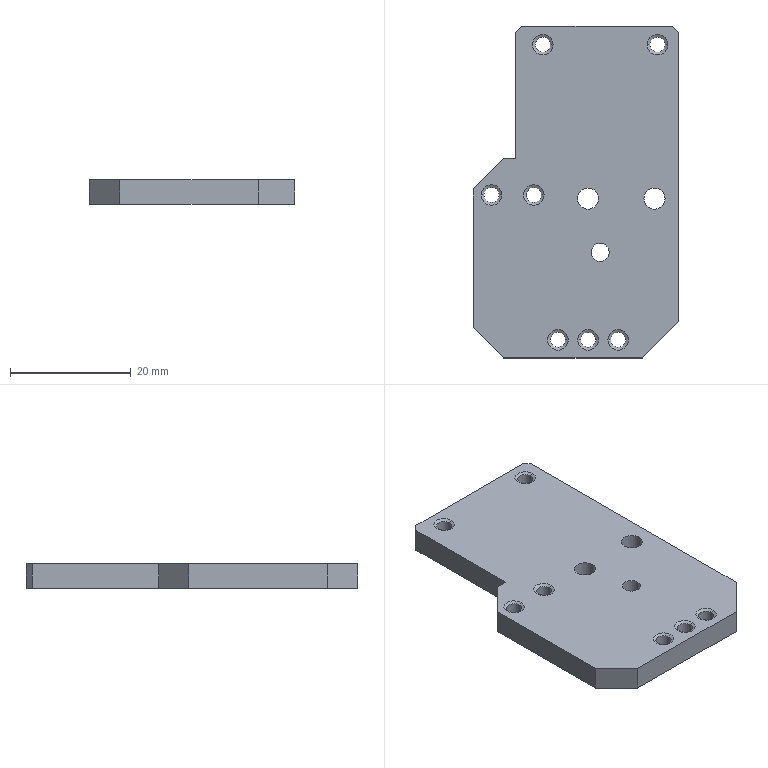Part | NX | 1 solid | 47 faces | box 34 x 55 x 4 mm | volume 6442 mm3 | cylinder 20 | cone 14 | plane 13 | commonest cylinder face diameters 2.5 x14 3.5 x4 3 x2
STEP:
#1=CARTESIAN_POINT('',(-9.5,5.5,2.));
#2=VERTEX_POINT('',#1);
#3=CARTESIAN_POINT('',(-11.5,5.5,2.));
#4=VERTEX_POINT('',#3);
#5=CARTESIAN_POINT('',(0.,5.5,2.));
#6=DIRECTION('',(-1.,0.,0.));
#7=VECTOR('',#6,1000.);
#8=LINE('',#5,#7);
#9=EDGE_CURVE('',#2,#4,#8,.T.);
#10=ORIENTED_EDGE('',*,*,#9,.T.);
#11=CARTESIAN_POINT('',(-16.5,0.5,2.));
#12=VERTEX_POINT('',#11);
#13=CARTESIAN_POINT('',(-17.,0.,2.));
#14=DIRECTION('',(-0.7071,-0.7071,0.));
#15=VECTOR('',#14,1000.);
#16=LINE('',#13,#15);
#17=EDGE_CURVE('',#4,#12,#16,.T.);
#18=ORIENTED_EDGE('',*,*,#17,.T.);
#19=CARTESIAN_POINT('',(-16.5,-22.5,2.));
#20=VERTEX_POINT('',#19);
#21=CARTESIAN_POINT('',(-16.5,0.,2.));
#22=DIRECTION('',(0.,-1.,0.));
#23=VECTOR('',#22,1000.);
#24=LINE('',#21,#23);
#25=EDGE_CURVE('',#12,#20,#24,.T.);
#26=ORIENTED_EDGE('',*,*,#25,.T.);
#27=CARTESIAN_POINT('',(-11.5,-27.5,2.));
#28=VERTEX_POINT('',#27);
#29=CARTESIAN_POINT('',(-39.,0.,2.));
#30=DIRECTION('',(-0.7071,0.7071,0.));
#31=VECTOR('',#30,1000.);
#32=LINE('',#29,#31);
#33=EDGE_CURVE('',#28,#20,#32,.T.);
#34=ORIENTED_EDGE('',*,*,#33,.F.);
#35=CARTESIAN_POINT('',(11.5,-27.5,2.));
#36=VERTEX_POINT('',#35);
#37=CARTESIAN_POINT('',(0.,-27.5,2.));
#38=DIRECTION('',(-1.,0.,0.));
#39=VECTOR('',#38,1000.);
#40=LINE('',#37,#39);
#41=EDGE_CURVE('',#36,#28,#40,.T.);
#42=ORIENTED_EDGE('',*,*,#41,.F.);
#43=CARTESIAN_POINT('',(17.5,-21.5,2.));
#44=VERTEX_POINT('',#43);
#45=CARTESIAN_POINT('',(39.,0.,2.));
#46=DIRECTION('',(-0.7071,-0.7071,0.));
#47=VECTOR('',#46,1000.);
#48=LINE('',#45,#47);
#49=EDGE_CURVE('',#44,#36,#48,.T.);
#50=ORIENTED_EDGE('',*,*,#49,.F.);
#51=CARTESIAN_POINT('',(17.5,26.5,2.));
#52=VERTEX_POINT('',#51);
#53=CARTESIAN_POINT('',(17.5,0.,2.));
#54=DIRECTION('',(0.,-1.,0.));
#55=VECTOR('',#54,1000.);
#56=LINE('',#53,#55);
#57=EDGE_CURVE('',#52,#44,#56,.T.);
#58=ORIENTED_EDGE('',*,*,#57,.F.);
#59=CARTESIAN_POINT('',(16.5,27.5,2.));
#60=VERTEX_POINT('',#59);
#61=CARTESIAN_POINT('',(44.,0.,2.));
#62=DIRECTION('',(0.7071,-0.7071,0.));
#63=VECTOR('',#62,1000.);
#64=LINE('',#61,#63);
#65=EDGE_CURVE('',#60,#52,#64,.T.);
#66=ORIENTED_EDGE('',*,*,#65,.F.);
#67=CARTESIAN_POINT('',(-8.5,27.5,2.));
#68=VERTEX_POINT('',#67);
#69=CARTESIAN_POINT('',(0.,27.5,2.));
#70=DIRECTION('',(1.,0.,0.));
#71=VECTOR('',#70,1000.);
#72=LINE('',#69,#71);
#73=EDGE_CURVE('',#68,#60,#72,.T.);
#74=ORIENTED_EDGE('',*,*,#73,.F.);
#75=CARTESIAN_POINT('',(-9.5,26.5,2.));
#76=VERTEX_POINT('',#75);
#77=CARTESIAN_POINT('',(-36.,0.,2.));
#78=DIRECTION('',(-0.7071,-0.7071,0.));
#79=VECTOR('',#78,1000.);
#80=LINE('',#77,#79);
#81=EDGE_CURVE('',#68,#76,#80,.T.);
#82=ORIENTED_EDGE('',*,*,#81,.T.);
#83=CARTESIAN_POINT('',(-9.5,0.,2.));
#84=DIRECTION('',(0.,-1.,0.));
#85=VECTOR('',#84,1000.);
#86=LINE('',#83,#85);
#87=EDGE_CURVE('',#76,#2,#86,.T.);
#88=ORIENTED_EDGE('',*,*,#87,.T.);
#89=EDGE_LOOP('',(#10,#18,#26,#34,#42,#50,#58,#66,#74,#82,#88));
#90=FACE_BOUND('',#89,.T.);
#91=CARTESIAN_POINT('',(15.25,-1.1,2.));
#92=VERTEX_POINT('',#91);
#93=CARTESIAN_POINT('',(11.75,-1.1,2.));
#94=VERTEX_POINT('',#93);
#95=CARTESIAN_POINT('',(13.5,-1.1,2.));
#96=DIRECTION('',(0.,0.,1.));
#97=DIRECTION('',(1.,0.,0.));
#98=AXIS2_PLACEMENT_3D('',#95,#96,#97);
#99=CIRCLE('',#98,1.75);
#100=EDGE_CURVE('',#92,#94,#99,.T.);
#101=ORIENTED_EDGE('',*,*,#100,.F.);
#102=CARTESIAN_POINT('',(13.5,-1.1,2.));
#103=DIRECTION('',(0.,0.,1.));
#104=DIRECTION('',(1.,0.,0.));
#105=AXIS2_PLACEMENT_3D('',#102,#103,#104);
#106=CIRCLE('',#105,1.75);
#107=EDGE_CURVE('',#94,#92,#106,.T.);
#108=ORIENTED_EDGE('',*,*,#107,.F.);
#109=EDGE_LOOP('',(#101,#108));
#110=FACE_BOUND('',#109,.T.);
#111=CARTESIAN_POINT('',(0.8,-24.5,2.));
#112=VERTEX_POINT('',#111);
#113=CARTESIAN_POINT('',(4.2,-24.5,2.));
#114=VERTEX_POINT('',#113);
#115=CARTESIAN_POINT('',(2.5,-24.5,2.));
#116=DIRECTION('',(0.,0.,1.));
#117=DIRECTION('',(1.,0.,0.));
#118=AXIS2_PLACEMENT_3D('',#115,#116,#117);
#119=CIRCLE('',#118,1.7);
#120=EDGE_CURVE('',#112,#114,#119,.T.);
#121=ORIENTED_EDGE('',*,*,#120,.F.);
#122=CARTESIAN_POINT('',(2.5,-24.5,2.));
#123=DIRECTION('',(0.,0.,1.));
#124=DIRECTION('',(1.,0.,0.));
#125=AXIS2_PLACEMENT_3D('',#122,#123,#124);
#126=CIRCLE('',#125,1.7);
#127=EDGE_CURVE('',#114,#112,#126,.T.);
#128=ORIENTED_EDGE('',*,*,#127,.F.);
#129=EDGE_LOOP('',(#121,#128));
#130=FACE_BOUND('',#129,.T.);
#131=CARTESIAN_POINT('',(-11.8,-0.5,2.));
#132=VERTEX_POINT('',#131);
#133=CARTESIAN_POINT('',(-15.2,-0.5,2.));
#134=VERTEX_POINT('',#133);
#135=CARTESIAN_POINT('',(-13.5,-0.5,2.));
#136=DIRECTION('',(0.,0.,1.));
#137=DIRECTION('',(1.,0.,0.));
#138=AXIS2_PLACEMENT_3D('',#135,#136,#137);
#139=CIRCLE('',#138,1.7);
#140=EDGE_CURVE('',#132,#134,#139,.T.);
#141=ORIENTED_EDGE('',*,*,#140,.F.);
#142=CARTESIAN_POINT('',(-13.5,-0.5,2.));
#143=DIRECTION('',(0.,0.,1.));
#144=DIRECTION('',(1.,0.,0.));
#145=AXIS2_PLACEMENT_3D('',#142,#143,#144);
#146=CIRCLE('',#145,1.7);
#147=EDGE_CURVE('',#134,#132,#146,.T.);
#148=ORIENTED_EDGE('',*,*,#147,.F.);
#149=EDGE_LOOP('',(#141,#148));
#150=FACE_BOUND('',#149,.T.);
#151=CARTESIAN_POINT('',(-6.7,24.4,2.));
#152=VERTEX_POINT('',#151);
#153=CARTESIAN_POINT('',(-3.3,24.4,2.));
#154=VERTEX_POINT('',#153);
#155=CARTESIAN_POINT('',(-5.,24.4,2.));
#156=DIRECTION('',(0.,0.,1.));
#157=DIRECTION('',(1.,0.,0.));
#158=AXIS2_PLACEMENT_3D('',#155,#156,#157);
#159=CIRCLE('',#158,1.7);
#160=EDGE_CURVE('',#152,#154,#159,.T.);
#161=ORIENTED_EDGE('',*,*,#160,.F.);
#162=CARTESIAN_POINT('',(-5.,24.4,2.));
#163=DIRECTION('',(0.,0.,1.));
#164=DIRECTION('',(1.,0.,0.));
#165=AXIS2_PLACEMENT_3D('',#162,#163,#164);
#166=CIRCLE('',#165,1.7);
#167=EDGE_CURVE('',#154,#152,#166,.T.);
#168=ORIENTED_EDGE('',*,*,#167,.F.);
#169=EDGE_LOOP('',(#161,#168));
#170=FACE_BOUND('',#169,.T.);
#171=CARTESIAN_POINT('',(4.25,-1.1,2.));
#172=VERTEX_POINT('',#171);
#173=CARTESIAN_POINT('',(0.75,-1.1,2.));
#174=VERTEX_POINT('',#173);
#175=CARTESIAN_POINT('',(2.5,-1.1,2.));
#176=DIRECTION('',(0.,0.,1.));
#177=DIRECTION('',(1.,0.,0.));
#178=AXIS2_PLACEMENT_3D('',#175,#176,#177);
#179=CIRCLE('',#178,1.75);
#180=EDGE_CURVE('',#172,#174,#179,.T.);
#181=ORIENTED_EDGE('',*,*,#180,.F.);
#182=CARTESIAN_POINT('',(2.5,-1.1,2.));
#183=DIRECTION('',(0.,0.,1.));
#184=DIRECTION('',(1.,0.,0.));
#185=AXIS2_PLACEMENT_3D('',#182,#183,#184);
#186=CIRCLE('',#185,1.75);
#187=EDGE_CURVE('',#174,#172,#186,.T.);
#188=ORIENTED_EDGE('',*,*,#187,.F.);
#189=EDGE_LOOP('',(#181,#188));
#190=FACE_BOUND('',#189,.T.);
#191=CARTESIAN_POINT('',(6.,-10.,2.));
#192=VERTEX_POINT('',#191);
#193=CARTESIAN_POINT('',(3.,-10.,2.));
#194=VERTEX_POINT('',#193);
#195=CARTESIAN_POINT('',(4.5,-10.,2.));
#196=DIRECTION('',(0.,0.,1.));
#197=DIRECTION('',(1.,0.,0.));
#198=AXIS2_PLACEMENT_3D('',#195,#196,#197);
#199=CIRCLE('',#198,1.5);
#200=EDGE_CURVE('',#192,#194,#199,.T.);
#201=ORIENTED_EDGE('',*,*,#200,.F.);
#202=CARTESIAN_POINT('',(4.5,-10.,2.));
#203=DIRECTION('',(0.,0.,1.));
#204=DIRECTION('',(1.,0.,0.));
#205=AXIS2_PLACEMENT_3D('',#202,#203,#204);
#206=CIRCLE('',#205,1.5);
#207=EDGE_CURVE('',#194,#192,#206,.T.);
#208=ORIENTED_EDGE('',*,*,#207,.F.);
#209=EDGE_LOOP('',(#201,#208));
#210=FACE_BOUND('',#209,.T.);
#211=CARTESIAN_POINT('',(12.3,24.4,2.));
#212=VERTEX_POINT('',#211);
#213=CARTESIAN_POINT('',(15.7,24.4,2.));
#214=VERTEX_POINT('',#213);
#215=CARTESIAN_POINT('',(14.,24.4,2.));
#216=DIRECTION('',(0.,0.,1.));
#217=DIRECTION('',(1.,0.,0.));
#218=AXIS2_PLACEMENT_3D('',#215,#216,#217);
#219=CIRCLE('',#218,1.7);
#220=EDGE_CURVE('',#212,#214,#219,.T.);
#221=ORIENTED_EDGE('',*,*,#220,.F.);
#222=CARTESIAN_POINT('',(14.,24.4,2.));
#223=DIRECTION('',(0.,0.,1.));
#224=DIRECTION('',(1.,0.,0.));
#225=AXIS2_PLACEMENT_3D('',#222,#223,#224);
#226=CIRCLE('',#225,1.7);
#227=EDGE_CURVE('',#214,#212,#226,.T.);
#228=ORIENTED_EDGE('',*,*,#227,.F.);
#229=EDGE_LOOP('',(#221,#228));
#230=FACE_BOUND('',#229,.T.);
#231=CARTESIAN_POINT('',(-4.8,-0.5,2.));
#232=VERTEX_POINT('',#231);
#233=CARTESIAN_POINT('',(-8.2,-0.5,2.));
#234=VERTEX_POINT('',#233);
#235=CARTESIAN_POINT('',(-6.5,-0.5,2.));
#236=DIRECTION('',(0.,0.,1.));
#237=DIRECTION('',(1.,0.,0.));
#238=AXIS2_PLACEMENT_3D('',#235,#236,#237);
#239=CIRCLE('',#238,1.7);
#240=EDGE_CURVE('',#232,#234,#239,.T.);
#241=ORIENTED_EDGE('',*,*,#240,.F.);
#242=CARTESIAN_POINT('',(-6.5,-0.5,2.));
#243=DIRECTION('',(0.,0.,1.));
#244=DIRECTION('',(1.,0.,0.));
#245=AXIS2_PLACEMENT_3D('',#242,#243,#244);
#246=CIRCLE('',#245,1.7);
#247=EDGE_CURVE('',#234,#232,#246,.T.);
#248=ORIENTED_EDGE('',*,*,#247,.F.);
#249=EDGE_LOOP('',(#241,#248));
#250=FACE_BOUND('',#249,.T.);
#251=CARTESIAN_POINT('',(-4.2,-24.5,2.));
#252=VERTEX_POINT('',#251);
#253=CARTESIAN_POINT('',(-0.8,-24.5,2.));
#254=VERTEX_POINT('',#253);
#255=CARTESIAN_POINT('',(-2.5,-24.5,2.));
#256=DIRECTION('',(0.,0.,1.));
#257=DIRECTION('',(1.,0.,0.));
#258=AXIS2_PLACEMENT_3D('',#255,#256,#257);
#259=CIRCLE('',#258,1.7);
#260=EDGE_CURVE('',#252,#254,#259,.T.);
#261=ORIENTED_EDGE('',*,*,#260,.F.);
#262=CARTESIAN_POINT('',(-2.5,-24.5,2.));
#263=DIRECTION('',(0.,0.,1.));
#264=DIRECTION('',(1.,0.,0.));
#265=AXIS2_PLACEMENT_3D('',#262,#263,#264);
#266=CIRCLE('',#265,1.7);
#267=EDGE_CURVE('',#254,#252,#266,.T.);
#268=ORIENTED_EDGE('',*,*,#267,.F.);
#269=EDGE_LOOP('',(#261,#268));
#270=FACE_BOUND('',#269,.T.);
#271=CARTESIAN_POINT('',(9.2,-24.5,2.));
#272=VERTEX_POINT('',#271);
#273=CARTESIAN_POINT('',(5.8,-24.5,2.));
#274=VERTEX_POINT('',#273);
#275=CARTESIAN_POINT('',(7.5,-24.5,2.));
#276=DIRECTION('',(0.,0.,1.));
#277=DIRECTION('',(1.,0.,0.));
#278=AXIS2_PLACEMENT_3D('',#275,#276,#277);
#279=CIRCLE('',#278,1.7);
#280=EDGE_CURVE('',#272,#274,#279,.T.);
#281=ORIENTED_EDGE('',*,*,#280,.F.);
#282=CARTESIAN_POINT('',(7.5,-24.5,2.));
#283=DIRECTION('',(0.,0.,1.));
#284=DIRECTION('',(1.,0.,0.));
#285=AXIS2_PLACEMENT_3D('',#282,#283,#284);
#286=CIRCLE('',#285,1.7);
#287=EDGE_CURVE('',#274,#272,#286,.T.);
#288=ORIENTED_EDGE('',*,*,#287,.F.);
#289=EDGE_LOOP('',(#281,#288));
#290=FACE_BOUND('',#289,.T.);
#291=CARTESIAN_POINT('',(0.,0.,2.));
#292=DIRECTION('',(0.,0.,1.));
#293=DIRECTION('',(1.,0.,0.));
#294=AXIS2_PLACEMENT_3D('',#291,#292,#293);
#295=PLANE('',#294);
#296=ADVANCED_FACE('',(#90,#110,#130,#150,#170,#190,#210,#230,#250,#270,#290),#295,.T.);
#297=CARTESIAN_POINT('',(-16.5,0.5,-2.));
#298=VERTEX_POINT('',#297);
#299=CARTESIAN_POINT('',(-16.5,0.5,0.));
#300=DIRECTION('',(0.,0.,1.));
#301=VECTOR('',#300,1000.);
#302=LINE('',#299,#301);
#303=EDGE_CURVE('',#298,#12,#302,.T.);
#304=ORIENTED_EDGE('',*,*,#303,.F.);
#305=CARTESIAN_POINT('',(-16.5,-22.5,-2.));
#306=VERTEX_POINT('',#305);
#307=CARTESIAN_POINT('',(-16.5,0.,-2.));
#308=DIRECTION('',(0.,-1.,0.));
#309=VECTOR('',#308,1000.);
#310=LINE('',#307,#309);
#311=EDGE_CURVE('',#298,#306,#310,.T.);
#312=ORIENTED_EDGE('',*,*,#311,.T.);
#313=CARTESIAN_POINT('',(-16.5,-22.5,0.));
#314=DIRECTION('',(0.,0.,1.));
#315=VECTOR('',#314,1000.);
#316=LINE('',#313,#315);
#317=EDGE_CURVE('',#306,#20,#316,.T.);
#318=ORIENTED_EDGE('',*,*,#317,.T.);
#319=ORIENTED_EDGE('',*,*,#25,.F.);
#320=EDGE_LOOP('',(#304,#312,#318,#319));
#321=FACE_BOUND('',#320,.T.);
#322=CARTESIAN_POINT('',(-16.5,3.686,-2.));
#323=DIRECTION('',(1.,0.,0.));
#324=DIRECTION('',(0.,1.,0.));
#325=AXIS2_PLACEMENT_3D('',#322,#323,#324);
#326=PLANE('',#325);
#327=ADVANCED_FACE('',(#321),#326,.F.);
#328=CARTESIAN_POINT('',(8.75,-24.5,-2.));
#329=VERTEX_POINT('',#328);
#330=CARTESIAN_POINT('',(6.25,-24.5,-2.));
#331=VERTEX_POINT('',#330);
#332=CARTESIAN_POINT('',(7.5,-24.5,-2.));
#333=DIRECTION('',(0.,0.,1.));
#334=DIRECTION('',(-1.,0.,0.));
#335=AXIS2_PLACEMENT_3D('',#332,#333,#334);
#336=CIRCLE('',#335,1.25);
#337=EDGE_CURVE('',#329,#331,#336,.T.);
#338=ORIENTED_EDGE('',*,*,#337,.F.);
#339=CARTESIAN_POINT('',(8.75,-24.5,1.74));
#340=VERTEX_POINT('',#339);
#341=CARTESIAN_POINT('',(8.75,-24.5,0.));
#342=DIRECTION('',(0.,0.,1.));
#343=VECTOR('',#342,1000.);
#344=LINE('',#341,#343);
#345=EDGE_CURVE('',#340,#329,#344,.F.);
#346=ORIENTED_EDGE('',*,*,#345,.F.);
#347=CARTESIAN_POINT('',(6.25,-24.5,1.74));
#348=VERTEX_POINT('',#347);
#349=CARTESIAN_POINT('',(7.5,-24.5,1.74));
#350=DIRECTION('',(0.,0.,1.));
#351=DIRECTION('',(1.,0.,0.));
#352=AXIS2_PLACEMENT_3D('',#349,#350,#351);
#353=CIRCLE('',#352,1.25);
#354=EDGE_CURVE('',#340,#348,#353,.T.);
#355=ORIENTED_EDGE('',*,*,#354,.T.);
#356=CARTESIAN_POINT('',(6.25,-24.5,0.));
#357=DIRECTION('',(0.,0.,1.));
#358=VECTOR('',#357,1000.);
#359=LINE('',#356,#358);
#360=EDGE_CURVE('',#348,#331,#359,.F.);
#361=ORIENTED_EDGE('',*,*,#360,.T.);
#362=EDGE_LOOP('',(#338,#346,#355,#361));
#363=FACE_BOUND('',#362,.T.);
#364=CARTESIAN_POINT('',(7.5,-24.5,0.));
#365=DIRECTION('',(0.,0.,1.));
#366=DIRECTION('',(-1.,0.,0.));
#367=AXIS2_PLACEMENT_3D('',#364,#365,#366);
#368=CYLINDRICAL_SURFACE('',#367,1.25);
#369=ADVANCED_FACE('',(#363),#368,.F.);
#370=CARTESIAN_POINT('',(-11.5,5.5,-2.));
#371=VERTEX_POINT('',#370);
#372=CARTESIAN_POINT('',(-11.5,5.5,0.));
#373=DIRECTION('',(0.,0.,-1.));
#374=VECTOR('',#373,1000.);
#375=LINE('',#372,#374);
#376=EDGE_CURVE('',#4,#371,#375,.T.);
#377=ORIENTED_EDGE('',*,*,#376,.F.);
#378=ORIENTED_EDGE('',*,*,#9,.F.);
#379=CARTESIAN_POINT('',(-9.5,5.5,-2.));
#380=VERTEX_POINT('',#379);
#381=CARTESIAN_POINT('',(-9.5,5.5,0.));
#382=DIRECTION('',(0.,0.,-1.));
#383=VECTOR('',#382,1000.);
#384=LINE('',#381,#383);
#385=EDGE_CURVE('',#2,#380,#384,.T.);
#386=ORIENTED_EDGE('',*,*,#385,.T.);
#387=CARTESIAN_POINT('',(0.,5.5,-2.));
#388=DIRECTION('',(-1.,0.,0.));
#389=VECTOR('',#388,1000.);
#390=LINE('',#387,#389);
#391=EDGE_CURVE('',#380,#371,#390,.T.);
#392=ORIENTED_EDGE('',*,*,#391,.T.);
#393=EDGE_LOOP('',(#377,#378,#386,#392));
#394=FACE_BOUND('',#393,.T.);
#395=CARTESIAN_POINT('',(-17.5,5.5,2.));
#396=DIRECTION('',(0.,-1.,0.));
#397=DIRECTION('',(0.,0.,-1.));
#398=AXIS2_PLACEMENT_3D('',#395,#396,#397);
#399=PLANE('',#398);
#400=ADVANCED_FACE('',(#394),#399,.F.);
#401=CARTESIAN_POINT('',(-9.5,26.5,-2.));
#402=VERTEX_POINT('',#401);
#403=CARTESIAN_POINT('',(-9.5,0.,-2.));
#404=DIRECTION('',(0.,-1.,0.));
#405=VECTOR('',#404,1000.);
#406=LINE('',#403,#405);
#407=EDGE_CURVE('',#402,#380,#406,.T.);
#408=ORIENTED_EDGE('',*,*,#407,.T.);
#409=ORIENTED_EDGE('',*,*,#385,.F.);
#410=ORIENTED_EDGE('',*,*,#87,.F.);
#411=CARTESIAN_POINT('',(-9.5,26.5,2.));
#412=DIRECTION('',(0.,0.,-1.));
#413=VECTOR('',#412,1000.);
#414=LINE('',#411,#413);
#415=EDGE_CURVE('',#76,#402,#414,.T.);
#416=ORIENTED_EDGE('',*,*,#415,.T.);
#417=EDGE_LOOP('',(#408,#409,#410,#416));
#418=FACE_BOUND('',#417,.T.);
#419=CARTESIAN_POINT('',(-9.5,5.5,2.));
#420=DIRECTION('',(1.,0.,0.));
#421=DIRECTION('',(0.,1.,0.));
#422=AXIS2_PLACEMENT_3D('',#419,#420,#421);
#423=PLANE('',#422);
#424=ADVANCED_FACE('',(#418),#423,.F.);
#425=CARTESIAN_POINT('',(-8.5,27.5,-2.));
#426=VERTEX_POINT('',#425);
#427=CARTESIAN_POINT('',(-8.5,27.5,2.));
#428=DIRECTION('',(0.,0.,-1.));
#429=VECTOR('',#428,1000.);
#430=LINE('',#427,#429);
#431=EDGE_CURVE('',#68,#426,#430,.T.);
#432=ORIENTED_EDGE('',*,*,#431,.T.);
#433=CARTESIAN_POINT('',(-36.,0.,-2.));
#434=DIRECTION('',(-0.7071,-0.7071,0.));
#435=VECTOR('',#434,1000.);
#436=LINE('',#433,#435);
#437=EDGE_CURVE('',#426,#402,#436,.T.);
#438=ORIENTED_EDGE('',*,*,#437,.T.);
#439=ORIENTED_EDGE('',*,*,#415,.F.);
#440=ORIENTED_EDGE('',*,*,#81,.F.);
#441=EDGE_LOOP('',(#432,#438,#439,#440));
#442=FACE_BOUND('',#441,.T.);
#443=CARTESIAN_POINT('',(-8.5,27.5,-2.));
#444=DIRECTION('',(0.7071,-0.7071,0.));
#445=DIRECTION('',(0.,0.,-1.));
#446=AXIS2_PLACEMENT_3D('',#443,#444,#445);
#447=PLANE('',#446);
#448=ADVANCED_FACE('',(#442),#447,.F.);
#449=ORIENTED_EDGE('',*,*,#431,.F.);
#450=ORIENTED_EDGE('',*,*,#73,.T.);
#451=CARTESIAN_POINT('',(16.5,27.5,-2.));
#452=VERTEX_POINT('',#451);
#453=CARTESIAN_POINT('',(16.5,27.5,2.));
#454=DIRECTION('',(0.,0.,-1.));
#455=VECTOR('',#454,1000.);
#456=LINE('',#453,#455);
#457=EDGE_CURVE('',#60,#452,#456,.T.);
#458=ORIENTED_EDGE('',*,*,#457,.T.);
#459=CARTESIAN_POINT('',(0.,27.5,-2.));
#460=DIRECTION('',(1.,0.,0.));
#461=VECTOR('',#460,1000.);
#462=LINE('',#459,#461);
#463=EDGE_CURVE('',#426,#452,#462,.T.);
#464=ORIENTED_EDGE('',*,*,#463,.F.);
#465=EDGE_LOOP('',(#449,#450,#458,#464));
#466=FACE_BOUND('',#465,.T.);
#467=CARTESIAN_POINT('',(17.5,27.5,-2.));
#468=DIRECTION('',(0.,1.,0.));
#469=DIRECTION('',(1.,0.,0.));
#470=AXIS2_PLACEMENT_3D('',#467,#468,#469);
#471=PLANE('',#470);
#472=ADVANCED_FACE('',(#466),#471,.T.);
#473=ORIENTED_EDGE('',*,*,#457,.F.);
#474=ORIENTED_EDGE('',*,*,#65,.T.);
#475=CARTESIAN_POINT('',(17.5,26.5,-2.));
#476=VERTEX_POINT('',#475);
#477=CARTESIAN_POINT('',(17.5,26.5,2.));
#478=DIRECTION('',(0.,0.,-1.));
#479=VECTOR('',#478,1000.);
#480=LINE('',#477,#479);
#481=EDGE_CURVE('',#52,#476,#480,.T.);
#482=ORIENTED_EDGE('',*,*,#481,.T.);
#483=CARTESIAN_POINT('',(44.,0.,-2.));
#484=DIRECTION('',(0.7071,-0.7071,0.));
#485=VECTOR('',#484,1000.);
#486=LINE('',#483,#485);
#487=EDGE_CURVE('',#452,#476,#486,.T.);
#488=ORIENTED_EDGE('',*,*,#487,.F.);
#489=EDGE_LOOP('',(#473,#474,#482,#488));
#490=FACE_BOUND('',#489,.T.);
#491=CARTESIAN_POINT('',(16.5,27.5,-2.));
#492=DIRECTION('',(0.7071,0.7071,0.));
#493=DIRECTION('',(0.,0.,-1.));
#494=AXIS2_PLACEMENT_3D('',#491,#492,#493);
#495=PLANE('',#494);
#496=ADVANCED_FACE('',(#490),#495,.T.);
#497=CARTESIAN_POINT('',(17.5,-21.5,-2.));
#498=VERTEX_POINT('',#497);
#499=CARTESIAN_POINT('',(17.5,0.,-2.));
#500=DIRECTION('',(0.,-1.,0.));
#501=VECTOR('',#500,1000.);
#502=LINE('',#499,#501);
#503=EDGE_CURVE('',#476,#498,#502,.T.);
#504=ORIENTED_EDGE('',*,*,#503,.F.);
#505=ORIENTED_EDGE('',*,*,#481,.F.);
#506=ORIENTED_EDGE('',*,*,#57,.T.);
#507=CARTESIAN_POINT('',(17.5,-21.5,2.));
#508=DIRECTION('',(0.,0.,-1.));
#509=VECTOR('',#508,1000.);
#510=LINE('',#507,#509);
#511=EDGE_CURVE('',#44,#498,#510,.T.);
#512=ORIENTED_EDGE('',*,*,#511,.T.);
#513=EDGE_LOOP('',(#504,#505,#506,#512));
#514=FACE_BOUND('',#513,.T.);
#515=CARTESIAN_POINT('',(17.5,-27.5,-2.));
#516=DIRECTION('',(1.,0.,0.));
#517=DIRECTION('',(0.,1.,0.));
#518=AXIS2_PLACEMENT_3D('',#515,#516,#517);
#519=PLANE('',#518);
#520=ADVANCED_FACE('',(#514),#519,.T.);
#521=ORIENTED_EDGE('',*,*,#511,.F.);
#522=ORIENTED_EDGE('',*,*,#49,.T.);
#523=CARTESIAN_POINT('',(11.5,-27.5,-2.));
#524=VERTEX_POINT('',#523);
#525=CARTESIAN_POINT('',(11.5,-27.5,2.));
#526=DIRECTION('',(0.,0.,-1.));
#527=VECTOR('',#526,1000.);
#528=LINE('',#525,#527);
#529=EDGE_CURVE('',#36,#524,#528,.T.);
#530=ORIENTED_EDGE('',*,*,#529,.T.);
#531=CARTESIAN_POINT('',(39.,0.,-2.));
#532=DIRECTION('',(-0.7071,-0.7071,0.));
#533=VECTOR('',#532,1000.);
#534=LINE('',#531,#533);
#535=EDGE_CURVE('',#498,#524,#534,.T.);
#536=ORIENTED_EDGE('',*,*,#535,.F.);
#537=EDGE_LOOP('',(#521,#522,#530,#536));
#538=FACE_BOUND('',#537,.T.);
#539=CARTESIAN_POINT('',(17.5,-21.5,-2.));
#540=DIRECTION('',(0.7071,-0.7071,0.));
#541=DIRECTION('',(0.,0.,-1.));
#542=AXIS2_PLACEMENT_3D('',#539,#540,#541);
#543=PLANE('',#542);
#544=ADVANCED_FACE('',(#538),#543,.T.);
#545=CARTESIAN_POINT('',(-11.5,-27.5,-2.));
#546=VERTEX_POINT('',#545);
#547=CARTESIAN_POINT('',(0.,-27.5,-2.));
#548=DIRECTION('',(-1.,0.,0.));
#549=VECTOR('',#548,1000.);
#550=LINE('',#547,#549);
#551=EDGE_CURVE('',#524,#546,#550,.T.);
#552=ORIENTED_EDGE('',*,*,#551,.F.);
#553=ORIENTED_EDGE('',*,*,#529,.F.);
#554=ORIENTED_EDGE('',*,*,#41,.T.);
#555=CARTESIAN_POINT('',(-11.5,-27.5,2.));
#556=DIRECTION('',(0.,0.,-1.));
#557=VECTOR('',#556,1000.);
#558=LINE('',#555,#557);
#559=EDGE_CURVE('',#28,#546,#558,.T.);
#560=ORIENTED_EDGE('',*,*,#559,.T.);
#561=EDGE_LOOP('',(#552,#553,#554,#560));
#562=FACE_BOUND('',#561,.T.);
#563=CARTESIAN_POINT('',(-17.5,-27.5,-2.));
#564=DIRECTION('',(0.,-1.,0.));
#565=DIRECTION('',(0.,0.,-1.));
#566=AXIS2_PLACEMENT_3D('',#563,#564,#565);
#567=PLANE('',#566);
#568=ADVANCED_FACE('',(#562),#567,.T.);
#569=ORIENTED_EDGE('',*,*,#317,.F.);
#570=CARTESIAN_POINT('',(-39.,0.,-2.));
#571=DIRECTION('',(-0.7071,0.7071,0.));
#572=VECTOR('',#571,1000.);
#573=LINE('',#570,#572);
#574=EDGE_CURVE('',#546,#306,#573,.T.);
#575=ORIENTED_EDGE('',*,*,#574,.F.);
#576=ORIENTED_EDGE('',*,*,#559,.F.);
#577=ORIENTED_EDGE('',*,*,#33,.T.);
#578=EDGE_LOOP('',(#569,#575,#576,#577));
#579=FACE_BOUND('',#578,.T.);
#580=CARTESIAN_POINT('',(-11.5,-27.5,-2.));
#581=DIRECTION('',(-0.7071,-0.7071,0.));
#582=DIRECTION('',(-0.7071,0.7071,0.));
#583=AXIS2_PLACEMENT_3D('',#580,#581,#582);
#584=PLANE('',#583);
#585=ADVANCED_FACE('',(#579),#584,.T.);
#586=ORIENTED_EDGE('',*,*,#311,.F.);
#587=CARTESIAN_POINT('',(-17.,0.,-2.));
#588=DIRECTION('',(-0.7071,-0.7071,0.));
#589=VECTOR('',#588,1000.);
#590=LINE('',#587,#589);
#591=EDGE_CURVE('',#371,#298,#590,.T.);
#592=ORIENTED_EDGE('',*,*,#591,.F.);
#593=ORIENTED_EDGE('',*,*,#391,.F.);
#594=ORIENTED_EDGE('',*,*,#407,.F.);
#595=ORIENTED_EDGE('',*,*,#437,.F.);
#596=ORIENTED_EDGE('',*,*,#463,.T.);
#597=ORIENTED_EDGE('',*,*,#487,.T.);
#598=ORIENTED_EDGE('',*,*,#503,.T.);
#599=ORIENTED_EDGE('',*,*,#535,.T.);
#600=ORIENTED_EDGE('',*,*,#551,.T.);
#601=ORIENTED_EDGE('',*,*,#574,.T.);
#602=EDGE_LOOP('',(#586,#592,#593,#594,#595,#596,#597,#598,#599,#600,#601));
#603=FACE_BOUND('',#602,.T.);
#604=CARTESIAN_POINT('',(11.75,-1.1,-2.));
#605=VERTEX_POINT('',#604);
#606=CARTESIAN_POINT('',(15.25,-1.1,-2.));
#607=VERTEX_POINT('',#606);
#608=CARTESIAN_POINT('',(13.5,-1.1,-2.));
#609=DIRECTION('',(0.,0.,1.));
#610=DIRECTION('',(1.,0.,0.));
#611=AXIS2_PLACEMENT_3D('',#608,#609,#610);
#612=CIRCLE('',#611,1.75);
#613=EDGE_CURVE('',#605,#607,#612,.T.);
#614=ORIENTED_EDGE('',*,*,#613,.T.);
#615=CARTESIAN_POINT('',(13.5,-1.1,-2.));
#616=DIRECTION('',(0.,0.,1.));
#617=DIRECTION('',(1.,0.,0.));
#618=AXIS2_PLACEMENT_3D('',#615,#616,#617);
#619=CIRCLE('',#618,1.75);
#620=EDGE_CURVE('',#607,#605,#619,.T.);
#621=ORIENTED_EDGE('',*,*,#620,.T.);
#622=EDGE_LOOP('',(#614,#621));
#623=FACE_BOUND('',#622,.T.);
#624=CARTESIAN_POINT('',(0.75,-1.1,-2.));
#625=VERTEX_POINT('',#624);
#626=CARTESIAN_POINT('',(4.25,-1.1,-2.));
#627=VERTEX_POINT('',#626);
#628=CARTESIAN_POINT('',(2.5,-1.1,-2.));
#629=DIRECTION('',(0.,0.,1.));
#630=DIRECTION('',(1.,0.,0.));
#631=AXIS2_PLACEMENT_3D('',#628,#629,#630);
#632=CIRCLE('',#631,1.75);
#633=EDGE_CURVE('',#625,#627,#632,.T.);
#634=ORIENTED_EDGE('',*,*,#633,.T.);
#635=CARTESIAN_POINT('',(2.5,-1.1,-2.));
#636=DIRECTION('',(0.,0.,1.));
#637=DIRECTION('',(1.,0.,0.));
#638=AXIS2_PLACEMENT_3D('',#635,#636,#637);
#639=CIRCLE('',#638,1.75);
#640=EDGE_CURVE('',#627,#625,#639,.T.);
#641=ORIENTED_EDGE('',*,*,#640,.T.);
#642=EDGE_LOOP('',(#634,#641));
#643=FACE_BOUND('',#642,.T.);
#644=CARTESIAN_POINT('',(3.,-10.,-2.));
#645=VERTEX_POINT('',#644);
#646=CARTESIAN_POINT('',(6.,-10.,-2.));
#647=VERTEX_POINT('',#646);
#648=CARTESIAN_POINT('',(4.5,-10.,-2.));
#649=DIRECTION('',(0.,0.,1.));
#650=DIRECTION('',(1.,0.,0.));
#651=AXIS2_PLACEMENT_3D('',#648,#649,#650);
#652=CIRCLE('',#651,1.5);
#653=EDGE_CURVE('',#645,#647,#652,.T.);
#654=ORIENTED_EDGE('',*,*,#653,.T.);
#655=CARTESIAN_POINT('',(4.5,-10.,-2.));
#656=DIRECTION('',(0.,0.,1.));
#657=DIRECTION('',(1.,0.,0.));
#658=AXIS2_PLACEMENT_3D('',#655,#656,#657);
#659=CIRCLE('',#658,1.5);
#660=EDGE_CURVE('',#647,#645,#659,.T.);
#661=ORIENTED_EDGE('',*,*,#660,.T.);
#662=EDGE_LOOP('',(#654,#661));
#663=FACE_BOUND('',#662,.T.);
#664=CARTESIAN_POINT('',(12.75,24.4,-2.));
#665=VERTEX_POINT('',#664);
#666=CARTESIAN_POINT('',(15.25,24.4,-2.));
#667=VERTEX_POINT('',#666);
#668=CARTESIAN_POINT('',(14.,24.4,-2.));
#669=DIRECTION('',(0.,0.,1.));
#670=DIRECTION('',(-1.,0.,0.));
#671=AXIS2_PLACEMENT_3D('',#668,#669,#670);
#672=CIRCLE('',#671,1.25);
#673=EDGE_CURVE('',#665,#667,#672,.T.);
#674=ORIENTED_EDGE('',*,*,#673,.T.);
#675=CARTESIAN_POINT('',(14.,24.4,-2.));
#676=DIRECTION('',(0.,0.,1.));
#677=DIRECTION('',(-1.,0.,0.));
#678=AXIS2_PLACEMENT_3D('',#675,#676,#677);
#679=CIRCLE('',#678,1.25);
#680=EDGE_CURVE('',#667,#665,#679,.T.);
#681=ORIENTED_EDGE('',*,*,#680,.T.);
#682=EDGE_LOOP('',(#674,#681));
#683=FACE_BOUND('',#682,.T.);
#684=CARTESIAN_POINT('',(-6.25,24.4,-2.));
#685=VERTEX_POINT('',#684);
#686=CARTESIAN_POINT('',(-3.75,24.4,-2.));
#687=VERTEX_POINT('',#686);
#688=CARTESIAN_POINT('',(-5.,24.4,-2.));
#689=DIRECTION('',(0.,0.,1.));
#690=DIRECTION('',(-1.,0.,0.));
#691=AXIS2_PLACEMENT_3D('',#688,#689,#690);
#692=CIRCLE('',#691,1.25);
#693=EDGE_CURVE('',#685,#687,#692,.T.);
#694=ORIENTED_EDGE('',*,*,#693,.T.);
#695=CARTESIAN_POINT('',(-5.,24.4,-2.));
#696=DIRECTION('',(0.,0.,1.));
#697=DIRECTION('',(-1.,0.,0.));
#698=AXIS2_PLACEMENT_3D('',#695,#696,#697);
#699=CIRCLE('',#698,1.25);
#700=EDGE_CURVE('',#687,#685,#699,.T.);
#701=ORIENTED_EDGE('',*,*,#700,.T.);
#702=EDGE_LOOP('',(#694,#701));
#703=FACE_BOUND('',#702,.T.);
#704=CARTESIAN_POINT('',(-5.25,-0.5,-2.));
#705=VERTEX_POINT('',#704);
#706=CARTESIAN_POINT('',(-7.75,-0.5,-2.));
#707=VERTEX_POINT('',#706);
#708=CARTESIAN_POINT('',(-6.5,-0.5,-2.));
#709=DIRECTION('',(0.,0.,1.));
#710=DIRECTION('',(-1.,0.,0.));
#711=AXIS2_PLACEMENT_3D('',#708,#709,#710);
#712=CIRCLE('',#711,1.25);
#713=EDGE_CURVE('',#705,#707,#712,.T.);
#714=ORIENTED_EDGE('',*,*,#713,.T.);
#715=CARTESIAN_POINT('',(-6.5,-0.5,-2.));
#716=DIRECTION('',(0.,0.,1.));
#717=DIRECTION('',(-1.,0.,0.));
#718=AXIS2_PLACEMENT_3D('',#715,#716,#717);
#719=CIRCLE('',#718,1.25);
#720=EDGE_CURVE('',#707,#705,#719,.T.);
#721=ORIENTED_EDGE('',*,*,#720,.T.);
#722=EDGE_LOOP('',(#714,#721));
#723=FACE_BOUND('',#722,.T.);
#724=CARTESIAN_POINT('',(-12.25,-0.5,-2.));
#725=VERTEX_POINT('',#724);
#726=CARTESIAN_POINT('',(-14.75,-0.5,-2.));
#727=VERTEX_POINT('',#726);
#728=CARTESIAN_POINT('',(-13.5,-0.5,-2.));
#729=DIRECTION('',(0.,0.,1.));
#730=DIRECTION('',(-1.,0.,0.));
#731=AXIS2_PLACEMENT_3D('',#728,#729,#730);
#732=CIRCLE('',#731,1.25);
#733=EDGE_CURVE('',#725,#727,#732,.T.);
#734=ORIENTED_EDGE('',*,*,#733,.T.);
#735=CARTESIAN_POINT('',(-13.5,-0.5,-2.));
#736=DIRECTION('',(0.,0.,1.));
#737=DIRECTION('',(-1.,0.,0.));
#738=AXIS2_PLACEMENT_3D('',#735,#736,#737);
#739=CIRCLE('',#738,1.25);
#740=EDGE_CURVE('',#727,#725,#739,.T.);
#741=ORIENTED_EDGE('',*,*,#740,.T.);
#742=EDGE_LOOP('',(#734,#741));
#743=FACE_BOUND('',#742,.T.);
#744=CARTESIAN_POINT('',(-1.25,-24.5,-2.));
#745=VERTEX_POINT('',#744);
#746=CARTESIAN_POINT('',(-3.75,-24.5,-2.));
#747=VERTEX_POINT('',#746);
#748=CARTESIAN_POINT('',(-2.5,-24.5,-2.));
#749=DIRECTION('',(0.,0.,1.));
#750=DIRECTION('',(-1.,0.,0.));
#751=AXIS2_PLACEMENT_3D('',#748,#749,#750);
#752=CIRCLE('',#751,1.25);
#753=EDGE_CURVE('',#745,#747,#752,.T.);
#754=ORIENTED_EDGE('',*,*,#753,.T.);
#755=CARTESIAN_POINT('',(-2.5,-24.5,-2.));
#756=DIRECTION('',(0.,0.,1.));
#757=DIRECTION('',(-1.,0.,0.));
#758=AXIS2_PLACEMENT_3D('',#755,#756,#757);
#759=CIRCLE('',#758,1.25);
#760=EDGE_CURVE('',#747,#745,#759,.T.);
#761=ORIENTED_EDGE('',*,*,#760,.T.);
#762=EDGE_LOOP('',(#754,#761));
#763=FACE_BOUND('',#762,.T.);
#764=CARTESIAN_POINT('',(3.75,-24.5,-2.));
#765=VERTEX_POINT('',#764);
#766=CARTESIAN_POINT('',(1.25,-24.5,-2.));
#767=VERTEX_POINT('',#766);
#768=CARTESIAN_POINT('',(2.5,-24.5,-2.));
#769=DIRECTION('',(0.,0.,1.));
#770=DIRECTION('',(-1.,0.,0.));
#771=AXIS2_PLACEMENT_3D('',#768,#769,#770);
#772=CIRCLE('',#771,1.25);
#773=EDGE_CURVE('',#765,#767,#772,.T.);
#774=ORIENTED_EDGE('',*,*,#773,.T.);
#775=CARTESIAN_POINT('',(2.5,-24.5,-2.));
#776=DIRECTION('',(0.,0.,1.));
#777=DIRECTION('',(-1.,0.,0.));
#778=AXIS2_PLACEMENT_3D('',#775,#776,#777);
#779=CIRCLE('',#778,1.25);
#780=EDGE_CURVE('',#767,#765,#779,.T.);
#781=ORIENTED_EDGE('',*,*,#780,.T.);
#782=EDGE_LOOP('',(#774,#781));
#783=FACE_BOUND('',#782,.T.);
#784=ORIENTED_EDGE('',*,*,#337,.T.);
#785=CARTESIAN_POINT('',(7.5,-24.5,-2.));
#786=DIRECTION('',(0.,0.,1.));
#787=DIRECTION('',(-1.,0.,0.));
#788=AXIS2_PLACEMENT_3D('',#785,#786,#787);
#789=CIRCLE('',#788,1.25);
#790=EDGE_CURVE('',#331,#329,#789,.T.);
#791=ORIENTED_EDGE('',*,*,#790,.T.);
#792=EDGE_LOOP('',(#784,#791));
#793=FACE_BOUND('',#792,.T.);
#794=CARTESIAN_POINT('',(0.,0.,-2.));
#795=DIRECTION('',(0.,0.,1.));
#796=DIRECTION('',(1.,0.,0.));
#797=AXIS2_PLACEMENT_3D('',#794,#795,#796);
#798=PLANE('',#797);
#799=ADVANCED_FACE('',(#603,#623,#643,#663,#683,#703,#723,#743,#763,#783,#793),#798,.F.);
#800=ORIENTED_EDGE('',*,*,#613,.F.);
#801=CARTESIAN_POINT('',(11.75,-1.1,-2.));
#802=DIRECTION('',(0.,0.,1.));
#803=VECTOR('',#802,1000.);
#804=LINE('',#801,#803);
#805=EDGE_CURVE('',#94,#605,#804,.F.);
#806=ORIENTED_EDGE('',*,*,#805,.F.);
#807=ORIENTED_EDGE('',*,*,#107,.T.);
#808=CARTESIAN_POINT('',(15.25,-1.1,-2.));
#809=DIRECTION('',(0.,0.,1.));
#810=VECTOR('',#809,1000.);
#811=LINE('',#808,#810);
#812=EDGE_CURVE('',#92,#607,#811,.F.);
#813=ORIENTED_EDGE('',*,*,#812,.T.);
#814=EDGE_LOOP('',(#800,#806,#807,#813));
#815=FACE_BOUND('',#814,.T.);
#816=CARTESIAN_POINT('',(13.5,-1.1,-2.));
#817=DIRECTION('',(0.,0.,1.));
#818=DIRECTION('',(1.,0.,0.));
#819=AXIS2_PLACEMENT_3D('',#816,#817,#818);
#820=CYLINDRICAL_SURFACE('',#819,1.75);
#821=ADVANCED_FACE('',(#815),#820,.F.);
#822=ORIENTED_EDGE('',*,*,#633,.F.);
#823=CARTESIAN_POINT('',(0.75,-1.1,-2.));
#824=DIRECTION('',(0.,0.,1.));
#825=VECTOR('',#824,1000.);
#826=LINE('',#823,#825);
#827=EDGE_CURVE('',#174,#625,#826,.F.);
#828=ORIENTED_EDGE('',*,*,#827,.F.);
#829=ORIENTED_EDGE('',*,*,#187,.T.);
#830=CARTESIAN_POINT('',(4.25,-1.1,-2.));
#831=DIRECTION('',(0.,0.,1.));
#832=VECTOR('',#831,1000.);
#833=LINE('',#830,#832);
#834=EDGE_CURVE('',#172,#627,#833,.F.);
#835=ORIENTED_EDGE('',*,*,#834,.T.);
#836=EDGE_LOOP('',(#822,#828,#829,#835));
#837=FACE_BOUND('',#836,.T.);
#838=CARTESIAN_POINT('',(2.5,-1.1,-2.));
#839=DIRECTION('',(0.,0.,1.));
#840=DIRECTION('',(1.,0.,0.));
#841=AXIS2_PLACEMENT_3D('',#838,#839,#840);
#842=CYLINDRICAL_SURFACE('',#841,1.75);
#843=ADVANCED_FACE('',(#837),#842,.F.);
#844=ORIENTED_EDGE('',*,*,#200,.T.);
#845=CARTESIAN_POINT('',(3.,-10.,-2.));
#846=DIRECTION('',(0.,0.,1.));
#847=VECTOR('',#846,1000.);
#848=LINE('',#845,#847);
#849=EDGE_CURVE('',#194,#645,#848,.F.);
#850=ORIENTED_EDGE('',*,*,#849,.T.);
#851=ORIENTED_EDGE('',*,*,#660,.F.);
#852=CARTESIAN_POINT('',(6.,-10.,-2.));
#853=DIRECTION('',(0.,0.,1.));
#854=VECTOR('',#853,1000.);
#855=LINE('',#852,#854);
#856=EDGE_CURVE('',#192,#647,#855,.F.);
#857=ORIENTED_EDGE('',*,*,#856,.F.);
#858=EDGE_LOOP('',(#844,#850,#851,#857));
#859=FACE_BOUND('',#858,.T.);
#860=CARTESIAN_POINT('',(4.5,-10.,-2.));
#861=DIRECTION('',(0.,0.,1.));
#862=DIRECTION('',(1.,0.,0.));
#863=AXIS2_PLACEMENT_3D('',#860,#861,#862);
#864=CYLINDRICAL_SURFACE('',#863,1.5);
#865=ADVANCED_FACE('',(#859),#864,.F.);
#866=ORIENTED_EDGE('',*,*,#673,.F.);
#867=CARTESIAN_POINT('',(12.75,24.4,1.74));
#868=VERTEX_POINT('',#867);
#869=CARTESIAN_POINT('',(12.75,24.4,0.));
#870=DIRECTION('',(0.,0.,1.));
#871=VECTOR('',#870,1000.);
#872=LINE('',#869,#871);
#873=EDGE_CURVE('',#868,#665,#872,.F.);
#874=ORIENTED_EDGE('',*,*,#873,.F.);
#875=CARTESIAN_POINT('',(15.25,24.4,1.74));
#876=VERTEX_POINT('',#875);
#877=CARTESIAN_POINT('',(14.,24.4,1.74));
#878=DIRECTION('',(0.,0.,1.));
#879=DIRECTION('',(1.,0.,0.));
#880=AXIS2_PLACEMENT_3D('',#877,#878,#879);
#881=CIRCLE('',#880,1.25);
#882=EDGE_CURVE('',#868,#876,#881,.T.);
#883=ORIENTED_EDGE('',*,*,#882,.T.);
#884=CARTESIAN_POINT('',(15.25,24.4,0.));
#885=DIRECTION('',(0.,0.,1.));
#886=VECTOR('',#885,1000.);
#887=LINE('',#884,#886);
#888=EDGE_CURVE('',#876,#667,#887,.F.);
#889=ORIENTED_EDGE('',*,*,#888,.T.);
#890=EDGE_LOOP('',(#866,#874,#883,#889));
#891=FACE_BOUND('',#890,.T.);
#892=CARTESIAN_POINT('',(14.,24.4,0.));
#893=DIRECTION('',(0.,0.,1.));
#894=DIRECTION('',(-1.,0.,0.));
#895=AXIS2_PLACEMENT_3D('',#892,#893,#894);
#896=CYLINDRICAL_SURFACE('',#895,1.25);
#897=ADVANCED_FACE('',(#891),#896,.F.);
#898=ORIENTED_EDGE('',*,*,#220,.T.);
#899=CARTESIAN_POINT('',(15.25,24.4,1.74));
#900=DIRECTION('',(0.866,0.,0.5));
#901=VECTOR('',#900,1000.);
#902=LINE('',#899,#901);
#903=EDGE_CURVE('',#876,#214,#902,.T.);
#904=ORIENTED_EDGE('',*,*,#903,.F.);
#905=ORIENTED_EDGE('',*,*,#882,.F.);
#906=CARTESIAN_POINT('',(12.75,24.4,1.74));
#907=DIRECTION('',(-0.866,0.,0.5));
#908=VECTOR('',#907,1000.);
#909=LINE('',#906,#908);
#910=EDGE_CURVE('',#868,#212,#909,.T.);
#911=ORIENTED_EDGE('',*,*,#910,.T.);
#912=EDGE_LOOP('',(#898,#904,#905,#911));
#913=FACE_BOUND('',#912,.T.);
#914=CARTESIAN_POINT('',(14.,24.4,1.74));
#915=DIRECTION('',(0.,0.,1.));
#916=DIRECTION('',(1.,0.,0.));
#917=AXIS2_PLACEMENT_3D('',#914,#915,#916);
#918=CONICAL_SURFACE('',#917,1.25,1.047);
#919=ADVANCED_FACE('',(#913),#918,.F.);
#920=ORIENTED_EDGE('',*,*,#693,.F.);
#921=CARTESIAN_POINT('',(-6.25,24.4,1.74));
#922=VERTEX_POINT('',#921);
#923=CARTESIAN_POINT('',(-6.25,24.4,0.));
#924=DIRECTION('',(0.,0.,1.));
#925=VECTOR('',#924,1000.);
#926=LINE('',#923,#925);
#927=EDGE_CURVE('',#922,#685,#926,.F.);
#928=ORIENTED_EDGE('',*,*,#927,.F.);
#929=CARTESIAN_POINT('',(-3.75,24.4,1.74));
#930=VERTEX_POINT('',#929);
#931=CARTESIAN_POINT('',(-5.,24.4,1.74));
#932=DIRECTION('',(0.,0.,1.));
#933=DIRECTION('',(1.,0.,0.));
#934=AXIS2_PLACEMENT_3D('',#931,#932,#933);
#935=CIRCLE('',#934,1.25);
#936=EDGE_CURVE('',#922,#930,#935,.T.);
#937=ORIENTED_EDGE('',*,*,#936,.T.);
#938=CARTESIAN_POINT('',(-3.75,24.4,0.));
#939=DIRECTION('',(0.,0.,1.));
#940=VECTOR('',#939,1000.);
#941=LINE('',#938,#940);
#942=EDGE_CURVE('',#930,#687,#941,.F.);
#943=ORIENTED_EDGE('',*,*,#942,.T.);
#944=EDGE_LOOP('',(#920,#928,#937,#943));
#945=FACE_BOUND('',#944,.T.);
#946=CARTESIAN_POINT('',(-5.,24.4,0.));
#947=DIRECTION('',(0.,0.,1.));
#948=DIRECTION('',(-1.,0.,0.));
#949=AXIS2_PLACEMENT_3D('',#946,#947,#948);
#950=CYLINDRICAL_SURFACE('',#949,1.25);
#951=ADVANCED_FACE('',(#945),#950,.F.);
#952=ORIENTED_EDGE('',*,*,#160,.T.);
#953=CARTESIAN_POINT('',(-3.75,24.4,1.74));
#954=DIRECTION('',(0.866,0.,0.5));
#955=VECTOR('',#954,1000.);
#956=LINE('',#953,#955);
#957=EDGE_CURVE('',#930,#154,#956,.T.);
#958=ORIENTED_EDGE('',*,*,#957,.F.);
#959=ORIENTED_EDGE('',*,*,#936,.F.);
#960=CARTESIAN_POINT('',(-6.25,24.4,1.74));
#961=DIRECTION('',(-0.866,0.,0.5));
#962=VECTOR('',#961,1000.);
#963=LINE('',#960,#962);
#964=EDGE_CURVE('',#922,#152,#963,.T.);
#965=ORIENTED_EDGE('',*,*,#964,.T.);
#966=EDGE_LOOP('',(#952,#958,#959,#965));
#967=FACE_BOUND('',#966,.T.);
#968=CARTESIAN_POINT('',(-5.,24.4,1.74));
#969=DIRECTION('',(0.,0.,1.));
#970=DIRECTION('',(1.,0.,0.));
#971=AXIS2_PLACEMENT_3D('',#968,#969,#970);
#972=CONICAL_SURFACE('',#971,1.25,1.047);
#973=ADVANCED_FACE('',(#967),#972,.F.);
#974=CARTESIAN_POINT('',(-7.75,-0.5,1.74));
#975=VERTEX_POINT('',#974);
#976=CARTESIAN_POINT('',(-5.25,-0.5,1.74));
#977=VERTEX_POINT('',#976);
#978=CARTESIAN_POINT('',(-6.5,-0.5,1.74));
#979=DIRECTION('',(0.,0.,1.));
#980=DIRECTION('',(1.,0.,0.));
#981=AXIS2_PLACEMENT_3D('',#978,#979,#980);
#982=CIRCLE('',#981,1.25);
#983=EDGE_CURVE('',#975,#977,#982,.T.);
#984=ORIENTED_EDGE('',*,*,#983,.T.);
#985=CARTESIAN_POINT('',(-5.25,-0.5,0.));
#986=DIRECTION('',(0.,0.,1.));
#987=VECTOR('',#986,1000.);
#988=LINE('',#985,#987);
#989=EDGE_CURVE('',#705,#977,#988,.T.);
#990=ORIENTED_EDGE('',*,*,#989,.F.);
#991=ORIENTED_EDGE('',*,*,#720,.F.);
#992=CARTESIAN_POINT('',(-7.75,-0.5,0.));
#993=DIRECTION('',(0.,0.,1.));
#994=VECTOR('',#993,1000.);
#995=LINE('',#992,#994);
#996=EDGE_CURVE('',#707,#975,#995,.T.);
#997=ORIENTED_EDGE('',*,*,#996,.T.);
#998=EDGE_LOOP('',(#984,#990,#991,#997));
#999=FACE_BOUND('',#998,.T.);
#1000=CARTESIAN_POINT('',(-6.5,-0.5,0.));
#1001=DIRECTION('',(0.,0.,1.));
#1002=DIRECTION('',(-1.,0.,0.));
#1003=AXIS2_PLACEMENT_3D('',#1000,#1001,#1002);
#1004=CYLINDRICAL_SURFACE('',#1003,1.25);
#1005=ADVANCED_FACE('',(#999),#1004,.F.);
#1006=ORIENTED_EDGE('',*,*,#240,.T.);
#1007=CARTESIAN_POINT('',(-7.75,-0.5,1.74));
#1008=DIRECTION('',(-0.866,0.,0.5));
#1009=VECTOR('',#1008,1000.);
#1010=LINE('',#1007,#1009);
#1011=EDGE_CURVE('',#234,#975,#1010,.F.);
#1012=ORIENTED_EDGE('',*,*,#1011,.T.);
#1013=CARTESIAN_POINT('',(-6.5,-0.5,1.74));
#1014=DIRECTION('',(0.,0.,1.));
#1015=DIRECTION('',(1.,0.,0.));
#1016=AXIS2_PLACEMENT_3D('',#1013,#1014,#1015);
#1017=CIRCLE('',#1016,1.25);
#1018=EDGE_CURVE('',#977,#975,#1017,.T.);
#1019=ORIENTED_EDGE('',*,*,#1018,.F.);
#1020=CARTESIAN_POINT('',(-5.25,-0.5,1.74));
#1021=DIRECTION('',(0.866,0.,0.5));
#1022=VECTOR('',#1021,1000.);
#1023=LINE('',#1020,#1022);
#1024=EDGE_CURVE('',#232,#977,#1023,.F.);
#1025=ORIENTED_EDGE('',*,*,#1024,.F.);
#1026=EDGE_LOOP('',(#1006,#1012,#1019,#1025));
#1027=FACE_BOUND('',#1026,.T.);
#1028=CARTESIAN_POINT('',(-6.5,-0.5,1.74));
#1029=DIRECTION('',(0.,0.,1.));
#1030=DIRECTION('',(1.,0.,0.));
#1031=AXIS2_PLACEMENT_3D('',#1028,#1029,#1030);
#1032=CONICAL_SURFACE('',#1031,1.25,1.047);
#1033=ADVANCED_FACE('',(#1027),#1032,.F.);
#1034=ORIENTED_EDGE('',*,*,#733,.F.);
#1035=CARTESIAN_POINT('',(-12.25,-0.5,1.74));
#1036=VERTEX_POINT('',#1035);
#1037=CARTESIAN_POINT('',(-12.25,-0.5,0.));
#1038=DIRECTION('',(0.,0.,1.));
#1039=VECTOR('',#1038,1000.);
#1040=LINE('',#1037,#1039);
#1041=EDGE_CURVE('',#725,#1036,#1040,.T.);
#1042=ORIENTED_EDGE('',*,*,#1041,.T.);
#1043=CARTESIAN_POINT('',(-14.75,-0.5,1.74));
#1044=VERTEX_POINT('',#1043);
#1045=CARTESIAN_POINT('',(-13.5,-0.5,1.74));
#1046=DIRECTION('',(0.,0.,1.));
#1047=DIRECTION('',(1.,0.,0.));
#1048=AXIS2_PLACEMENT_3D('',#1045,#1046,#1047);
#1049=CIRCLE('',#1048,1.25);
#1050=EDGE_CURVE('',#1036,#1044,#1049,.T.);
#1051=ORIENTED_EDGE('',*,*,#1050,.T.);
#1052=CARTESIAN_POINT('',(-14.75,-0.5,0.));
#1053=DIRECTION('',(0.,0.,1.));
#1054=VECTOR('',#1053,1000.);
#1055=LINE('',#1052,#1054);
#1056=EDGE_CURVE('',#727,#1044,#1055,.T.);
#1057=ORIENTED_EDGE('',*,*,#1056,.F.);
#1058=EDGE_LOOP('',(#1034,#1042,#1051,#1057));
#1059=FACE_BOUND('',#1058,.T.);
#1060=CARTESIAN_POINT('',(-13.5,-0.5,0.));
#1061=DIRECTION('',(0.,0.,1.));
#1062=DIRECTION('',(-1.,0.,0.));
#1063=AXIS2_PLACEMENT_3D('',#1060,#1061,#1062);
#1064=CYLINDRICAL_SURFACE('',#1063,1.25);
#1065=ADVANCED_FACE('',(#1059),#1064,.F.);
#1066=ORIENTED_EDGE('',*,*,#140,.T.);
#1067=CARTESIAN_POINT('',(-15.2,-0.5,2.));
#1068=DIRECTION('',(-0.866,0.,0.5));
#1069=VECTOR('',#1068,1000.);
#1070=LINE('',#1067,#1069);
#1071=EDGE_CURVE('',#134,#1044,#1070,.F.);
#1072=ORIENTED_EDGE('',*,*,#1071,.T.);
#1073=ORIENTED_EDGE('',*,*,#1050,.F.);
#1074=CARTESIAN_POINT('',(-11.8,-0.5,2.));
#1075=DIRECTION('',(0.866,0.,0.5));
#1076=VECTOR('',#1075,1000.);
#1077=LINE('',#1074,#1076);
#1078=EDGE_CURVE('',#132,#1036,#1077,.F.);
#1079=ORIENTED_EDGE('',*,*,#1078,.F.);
#1080=EDGE_LOOP('',(#1066,#1072,#1073,#1079));
#1081=FACE_BOUND('',#1080,.T.);
#1082=CARTESIAN_POINT('',(-13.5,-0.5,2.));
#1083=DIRECTION('',(0.,0.,1.));
#1084=DIRECTION('',(1.,0.,0.));
#1085=AXIS2_PLACEMENT_3D('',#1082,#1083,#1084);
#1086=CONICAL_SURFACE('',#1085,1.7,1.047);
#1087=ADVANCED_FACE('',(#1081),#1086,.F.);
#1088=CARTESIAN_POINT('',(-3.75,-24.5,1.74));
#1089=VERTEX_POINT('',#1088);
#1090=CARTESIAN_POINT('',(-1.25,-24.5,1.74));
#1091=VERTEX_POINT('',#1090);
#1092=CARTESIAN_POINT('',(-2.5,-24.5,1.74));
#1093=DIRECTION('',(0.,0.,1.));
#1094=DIRECTION('',(1.,0.,0.));
#1095=AXIS2_PLACEMENT_3D('',#1092,#1093,#1094);
#1096=CIRCLE('',#1095,1.25);
#1097=EDGE_CURVE('',#1089,#1091,#1096,.T.);
#1098=ORIENTED_EDGE('',*,*,#1097,.T.);
#1099=CARTESIAN_POINT('',(-1.25,-24.5,0.));
#1100=DIRECTION('',(0.,0.,1.));
#1101=VECTOR('',#1100,1000.);
#1102=LINE('',#1099,#1101);
#1103=EDGE_CURVE('',#745,#1091,#1102,.T.);
#1104=ORIENTED_EDGE('',*,*,#1103,.F.);
#1105=ORIENTED_EDGE('',*,*,#760,.F.);
#1106=CARTESIAN_POINT('',(-3.75,-24.5,0.));
#1107=DIRECTION('',(0.,0.,1.));
#1108=VECTOR('',#1107,1000.);
#1109=LINE('',#1106,#1108);
#1110=EDGE_CURVE('',#747,#1089,#1109,.T.);
#1111=ORIENTED_EDGE('',*,*,#1110,.T.);
#1112=EDGE_LOOP('',(#1098,#1104,#1105,#1111));
#1113=FACE_BOUND('',#1112,.T.);
#1114=CARTESIAN_POINT('',(-2.5,-24.5,0.));
#1115=DIRECTION('',(0.,0.,1.));
#1116=DIRECTION('',(-1.,0.,0.));
#1117=AXIS2_PLACEMENT_3D('',#1114,#1115,#1116);
#1118=CYLINDRICAL_SURFACE('',#1117,1.25);
#1119=ADVANCED_FACE('',(#1113),#1118,.F.);
#1120=ORIENTED_EDGE('',*,*,#303,.T.);
#1121=ORIENTED_EDGE('',*,*,#17,.F.);
#1122=ORIENTED_EDGE('',*,*,#376,.T.);
#1123=ORIENTED_EDGE('',*,*,#591,.T.);
#1124=EDGE_LOOP('',(#1120,#1121,#1122,#1123));
#1125=FACE_BOUND('',#1124,.T.);
#1126=CARTESIAN_POINT('',(-14.,3.,0.));
#1127=DIRECTION('',(0.7071,-0.7071,0.));
#1128=DIRECTION('',(0.,0.,-1.));
#1129=AXIS2_PLACEMENT_3D('',#1126,#1127,#1128);
#1130=PLANE('',#1129);
#1131=ADVANCED_FACE('',(#1125),#1130,.F.);
#1132=CARTESIAN_POINT('',(1.25,-24.5,1.74));
#1133=VERTEX_POINT('',#1132);
#1134=CARTESIAN_POINT('',(3.75,-24.5,1.74));
#1135=VERTEX_POINT('',#1134);
#1136=CARTESIAN_POINT('',(2.5,-24.5,1.74));
#1137=DIRECTION('',(0.,0.,1.));
#1138=DIRECTION('',(1.,0.,0.));
#1139=AXIS2_PLACEMENT_3D('',#1136,#1137,#1138);
#1140=CIRCLE('',#1139,1.25);
#1141=EDGE_CURVE('',#1133,#1135,#1140,.T.);
#1142=ORIENTED_EDGE('',*,*,#1141,.T.);
#1143=CARTESIAN_POINT('',(3.75,-24.5,0.));
#1144=DIRECTION('',(0.,0.,1.));
#1145=VECTOR('',#1144,1000.);
#1146=LINE('',#1143,#1145);
#1147=EDGE_CURVE('',#765,#1135,#1146,.T.);
#1148=ORIENTED_EDGE('',*,*,#1147,.F.);
#1149=ORIENTED_EDGE('',*,*,#780,.F.);
#1150=CARTESIAN_POINT('',(1.25,-24.5,0.));
#1151=DIRECTION('',(0.,0.,1.));
#1152=VECTOR('',#1151,1000.);
#1153=LINE('',#1150,#1152);
#1154=EDGE_CURVE('',#767,#1133,#1153,.T.);
#1155=ORIENTED_EDGE('',*,*,#1154,.T.);
#1156=EDGE_LOOP('',(#1142,#1148,#1149,#1155));
#1157=FACE_BOUND('',#1156,.T.);
#1158=CARTESIAN_POINT('',(2.5,-24.5,0.));
#1159=DIRECTION('',(0.,0.,1.));
#1160=DIRECTION('',(-1.,0.,0.));
#1161=AXIS2_PLACEMENT_3D('',#1158,#1159,#1160);
#1162=CYLINDRICAL_SURFACE('',#1161,1.25);
#1163=ADVANCED_FACE('',(#1157),#1162,.F.);
#1164=ORIENTED_EDGE('',*,*,#1097,.F.);
#1165=CARTESIAN_POINT('',(-4.2,-24.5,2.));
#1166=DIRECTION('',(-0.866,0.,0.5));
#1167=VECTOR('',#1166,1000.);
#1168=LINE('',#1165,#1167);
#1169=EDGE_CURVE('',#1089,#252,#1168,.T.);
#1170=ORIENTED_EDGE('',*,*,#1169,.T.);
#1171=ORIENTED_EDGE('',*,*,#260,.T.);
#1172=CARTESIAN_POINT('',(-0.8,-24.5,2.));
#1173=DIRECTION('',(0.866,0.,0.5));
#1174=VECTOR('',#1173,1000.);
#1175=LINE('',#1172,#1174);
#1176=EDGE_CURVE('',#1091,#254,#1175,.T.);
#1177=ORIENTED_EDGE('',*,*,#1176,.F.);
#1178=EDGE_LOOP('',(#1164,#1170,#1171,#1177));
#1179=FACE_BOUND('',#1178,.T.);
#1180=CARTESIAN_POINT('',(-2.5,-24.5,2.));
#1181=DIRECTION('',(0.,0.,1.));
#1182=DIRECTION('',(1.,0.,0.));
#1183=AXIS2_PLACEMENT_3D('',#1180,#1181,#1182);
#1184=CONICAL_SURFACE('',#1183,1.7,1.047);
#1185=ADVANCED_FACE('',(#1179),#1184,.F.);
#1186=ORIENTED_EDGE('',*,*,#354,.F.);
#1187=CARTESIAN_POINT('',(9.2,-24.5,2.));
#1188=DIRECTION('',(0.866,0.,0.5));
#1189=VECTOR('',#1188,1000.);
#1190=LINE('',#1187,#1189);
#1191=EDGE_CURVE('',#340,#272,#1190,.T.);
#1192=ORIENTED_EDGE('',*,*,#1191,.T.);
#1193=ORIENTED_EDGE('',*,*,#280,.T.);
#1194=CARTESIAN_POINT('',(5.8,-24.5,2.));
#1195=DIRECTION('',(-0.866,0.,0.5));
#1196=VECTOR('',#1195,1000.);
#1197=LINE('',#1194,#1196);
#1198=EDGE_CURVE('',#348,#274,#1197,.T.);
#1199=ORIENTED_EDGE('',*,*,#1198,.F.);
#1200=EDGE_LOOP('',(#1186,#1192,#1193,#1199));
#1201=FACE_BOUND('',#1200,.T.);
#1202=CARTESIAN_POINT('',(7.5,-24.5,2.));
#1203=DIRECTION('',(0.,0.,1.));
#1204=DIRECTION('',(1.,0.,0.));
#1205=AXIS2_PLACEMENT_3D('',#1202,#1203,#1204);
#1206=CONICAL_SURFACE('',#1205,1.7,1.047);
#1207=ADVANCED_FACE('',(#1201),#1206,.F.);
#1208=ORIENTED_EDGE('',*,*,#1141,.F.);
#1209=CARTESIAN_POINT('',(1.25,-24.5,1.74));
#1210=DIRECTION('',(-0.866,0.,0.5));
#1211=VECTOR('',#1210,1000.);
#1212=LINE('',#1209,#1211);
#1213=EDGE_CURVE('',#1133,#112,#1212,.T.);
#1214=ORIENTED_EDGE('',*,*,#1213,.T.);
#1215=ORIENTED_EDGE('',*,*,#120,.T.);
#1216=CARTESIAN_POINT('',(3.75,-24.5,1.74));
#1217=DIRECTION('',(0.866,0.,0.5));
#1218=VECTOR('',#1217,1000.);
#1219=LINE('',#1216,#1218);
#1220=EDGE_CURVE('',#1135,#114,#1219,.T.);
#1221=ORIENTED_EDGE('',*,*,#1220,.F.);
#1222=EDGE_LOOP('',(#1208,#1214,#1215,#1221));
#1223=FACE_BOUND('',#1222,.T.);
#1224=CARTESIAN_POINT('',(2.5,-24.5,1.74));
#1225=DIRECTION('',(0.,0.,1.));
#1226=DIRECTION('',(1.,0.,0.));
#1227=AXIS2_PLACEMENT_3D('',#1224,#1225,#1226);
#1228=CONICAL_SURFACE('',#1227,1.25,1.047);
#1229=ADVANCED_FACE('',(#1223),#1228,.F.);
#1230=ORIENTED_EDGE('',*,*,#100,.T.);
#1231=ORIENTED_EDGE('',*,*,#805,.T.);
#1232=ORIENTED_EDGE('',*,*,#620,.F.);
#1233=ORIENTED_EDGE('',*,*,#812,.F.);
#1234=EDGE_LOOP('',(#1230,#1231,#1232,#1233));
#1235=FACE_BOUND('',#1234,.T.);
#1236=CARTESIAN_POINT('',(13.5,-1.1,-2.));
#1237=DIRECTION('',(0.,0.,1.));
#1238=DIRECTION('',(1.,0.,0.));
#1239=AXIS2_PLACEMENT_3D('',#1236,#1237,#1238);
#1240=CYLINDRICAL_SURFACE('',#1239,1.75);
#1241=ADVANCED_FACE('',(#1235),#1240,.F.);
#1242=ORIENTED_EDGE('',*,*,#1191,.F.);
#1243=CARTESIAN_POINT('',(7.5,-24.5,1.74));
#1244=DIRECTION('',(0.,0.,1.));
#1245=DIRECTION('',(1.,0.,0.));
#1246=AXIS2_PLACEMENT_3D('',#1243,#1244,#1245);
#1247=CIRCLE('',#1246,1.25);
#1248=EDGE_CURVE('',#348,#340,#1247,.T.);
#1249=ORIENTED_EDGE('',*,*,#1248,.F.);
#1250=ORIENTED_EDGE('',*,*,#1198,.T.);
#1251=ORIENTED_EDGE('',*,*,#287,.T.);
#1252=EDGE_LOOP('',(#1242,#1249,#1250,#1251));
#1253=FACE_BOUND('',#1252,.T.);
#1254=CARTESIAN_POINT('',(7.5,-24.5,2.));
#1255=DIRECTION('',(0.,0.,1.));
#1256=DIRECTION('',(1.,0.,0.));
#1257=AXIS2_PLACEMENT_3D('',#1254,#1255,#1256);
#1258=CONICAL_SURFACE('',#1257,1.7,1.047);
#1259=ADVANCED_FACE('',(#1253),#1258,.F.);
#1260=ORIENTED_EDGE('',*,*,#773,.F.);
#1261=ORIENTED_EDGE('',*,*,#1147,.T.);
#1262=CARTESIAN_POINT('',(2.5,-24.5,1.74));
#1263=DIRECTION('',(0.,0.,1.));
#1264=DIRECTION('',(1.,0.,0.));
#1265=AXIS2_PLACEMENT_3D('',#1262,#1263,#1264);
#1266=CIRCLE('',#1265,1.25);
#1267=EDGE_CURVE('',#1135,#1133,#1266,.T.);
#1268=ORIENTED_EDGE('',*,*,#1267,.T.);
#1269=ORIENTED_EDGE('',*,*,#1154,.F.);
#1270=EDGE_LOOP('',(#1260,#1261,#1268,#1269));
#1271=FACE_BOUND('',#1270,.T.);
#1272=CARTESIAN_POINT('',(2.5,-24.5,0.));
#1273=DIRECTION('',(0.,0.,1.));
#1274=DIRECTION('',(-1.,0.,0.));
#1275=AXIS2_PLACEMENT_3D('',#1272,#1273,#1274);
#1276=CYLINDRICAL_SURFACE('',#1275,1.25);
#1277=ADVANCED_FACE('',(#1271),#1276,.F.);
#1278=CARTESIAN_POINT('',(-13.5,-0.5,1.74));
#1279=DIRECTION('',(0.,0.,1.));
#1280=DIRECTION('',(1.,0.,0.));
#1281=AXIS2_PLACEMENT_3D('',#1278,#1279,#1280);
#1282=CIRCLE('',#1281,1.25);
#1283=EDGE_CURVE('',#1044,#1036,#1282,.T.);
#1284=ORIENTED_EDGE('',*,*,#1283,.F.);
#1285=ORIENTED_EDGE('',*,*,#1071,.F.);
#1286=ORIENTED_EDGE('',*,*,#147,.T.);
#1287=ORIENTED_EDGE('',*,*,#1078,.T.);
#1288=EDGE_LOOP('',(#1284,#1285,#1286,#1287));
#1289=FACE_BOUND('',#1288,.T.);
#1290=CARTESIAN_POINT('',(-13.5,-0.5,2.));
#1291=DIRECTION('',(0.,0.,1.));
#1292=DIRECTION('',(1.,0.,0.));
#1293=AXIS2_PLACEMENT_3D('',#1290,#1291,#1292);
#1294=CONICAL_SURFACE('',#1293,1.7,1.047);
#1295=ADVANCED_FACE('',(#1289),#1294,.F.);
#1296=ORIENTED_EDGE('',*,*,#713,.F.);
#1297=ORIENTED_EDGE('',*,*,#989,.T.);
#1298=ORIENTED_EDGE('',*,*,#1018,.T.);
#1299=ORIENTED_EDGE('',*,*,#996,.F.);
#1300=EDGE_LOOP('',(#1296,#1297,#1298,#1299));
#1301=FACE_BOUND('',#1300,.T.);
#1302=CARTESIAN_POINT('',(-6.5,-0.5,0.));
#1303=DIRECTION('',(0.,0.,1.));
#1304=DIRECTION('',(-1.,0.,0.));
#1305=AXIS2_PLACEMENT_3D('',#1302,#1303,#1304);
#1306=CYLINDRICAL_SURFACE('',#1305,1.25);
#1307=ADVANCED_FACE('',(#1301),#1306,.F.);
#1308=CARTESIAN_POINT('',(14.,24.4,1.74));
#1309=DIRECTION('',(0.,0.,1.));
#1310=DIRECTION('',(1.,0.,0.));
#1311=AXIS2_PLACEMENT_3D('',#1308,#1309,#1310);
#1312=CIRCLE('',#1311,1.25);
#1313=EDGE_CURVE('',#876,#868,#1312,.T.);
#1314=ORIENTED_EDGE('',*,*,#1313,.F.);
#1315=ORIENTED_EDGE('',*,*,#903,.T.);
#1316=ORIENTED_EDGE('',*,*,#227,.T.);
#1317=ORIENTED_EDGE('',*,*,#910,.F.);
#1318=EDGE_LOOP('',(#1314,#1315,#1316,#1317));
#1319=FACE_BOUND('',#1318,.T.);
#1320=CARTESIAN_POINT('',(14.,24.4,1.74));
#1321=DIRECTION('',(0.,0.,1.));
#1322=DIRECTION('',(1.,0.,0.));
#1323=AXIS2_PLACEMENT_3D('',#1320,#1321,#1322);
#1324=CONICAL_SURFACE('',#1323,1.25,1.047);
#1325=ADVANCED_FACE('',(#1319),#1324,.F.);
#1326=ORIENTED_EDGE('',*,*,#180,.T.);
#1327=ORIENTED_EDGE('',*,*,#827,.T.);
#1328=ORIENTED_EDGE('',*,*,#640,.F.);
#1329=ORIENTED_EDGE('',*,*,#834,.F.);
#1330=EDGE_LOOP('',(#1326,#1327,#1328,#1329));
#1331=FACE_BOUND('',#1330,.T.);
#1332=CARTESIAN_POINT('',(2.5,-1.1,-2.));
#1333=DIRECTION('',(0.,0.,1.));
#1334=DIRECTION('',(1.,0.,0.));
#1335=AXIS2_PLACEMENT_3D('',#1332,#1333,#1334);
#1336=CYLINDRICAL_SURFACE('',#1335,1.75);
#1337=ADVANCED_FACE('',(#1331),#1336,.F.);
#1338=ORIENTED_EDGE('',*,*,#1220,.T.);
#1339=ORIENTED_EDGE('',*,*,#127,.T.);
#1340=ORIENTED_EDGE('',*,*,#1213,.F.);
#1341=ORIENTED_EDGE('',*,*,#1267,.F.);
#1342=EDGE_LOOP('',(#1338,#1339,#1340,#1341));
#1343=FACE_BOUND('',#1342,.T.);
#1344=CARTESIAN_POINT('',(2.5,-24.5,1.74));
#1345=DIRECTION('',(0.,0.,1.));
#1346=DIRECTION('',(1.,0.,0.));
#1347=AXIS2_PLACEMENT_3D('',#1344,#1345,#1346);
#1348=CONICAL_SURFACE('',#1347,1.25,1.047);
#1349=ADVANCED_FACE('',(#1343),#1348,.F.);
#1350=ORIENTED_EDGE('',*,*,#753,.F.);
#1351=ORIENTED_EDGE('',*,*,#1103,.T.);
#1352=CARTESIAN_POINT('',(-2.5,-24.5,1.74));
#1353=DIRECTION('',(0.,0.,1.));
#1354=DIRECTION('',(1.,0.,0.));
#1355=AXIS2_PLACEMENT_3D('',#1352,#1353,#1354);
#1356=CIRCLE('',#1355,1.25);
#1357=EDGE_CURVE('',#1091,#1089,#1356,.T.);
#1358=ORIENTED_EDGE('',*,*,#1357,.T.);
#1359=ORIENTED_EDGE('',*,*,#1110,.F.);
#1360=EDGE_LOOP('',(#1350,#1351,#1358,#1359));
#1361=FACE_BOUND('',#1360,.T.);
#1362=CARTESIAN_POINT('',(-2.5,-24.5,0.));
#1363=DIRECTION('',(0.,0.,1.));
#1364=DIRECTION('',(-1.,0.,0.));
#1365=AXIS2_PLACEMENT_3D('',#1362,#1363,#1364);
#1366=CYLINDRICAL_SURFACE('',#1365,1.25);
#1367=ADVANCED_FACE('',(#1361),#1366,.F.);
#1368=ORIENTED_EDGE('',*,*,#983,.F.);
#1369=ORIENTED_EDGE('',*,*,#1011,.F.);
#1370=ORIENTED_EDGE('',*,*,#247,.T.);
#1371=ORIENTED_EDGE('',*,*,#1024,.T.);
#1372=EDGE_LOOP('',(#1368,#1369,#1370,#1371));
#1373=FACE_BOUND('',#1372,.T.);
#1374=CARTESIAN_POINT('',(-6.5,-0.5,1.74));
#1375=DIRECTION('',(0.,0.,1.));
#1376=DIRECTION('',(1.,0.,0.));
#1377=AXIS2_PLACEMENT_3D('',#1374,#1375,#1376);
#1378=CONICAL_SURFACE('',#1377,1.25,1.047);
#1379=ADVANCED_FACE('',(#1373),#1378,.F.);
#1380=CARTESIAN_POINT('',(-5.,24.4,1.74));
#1381=DIRECTION('',(0.,0.,1.));
#1382=DIRECTION('',(1.,0.,0.));
#1383=AXIS2_PLACEMENT_3D('',#1380,#1381,#1382);
#1384=CIRCLE('',#1383,1.25);
#1385=EDGE_CURVE('',#930,#922,#1384,.T.);
#1386=ORIENTED_EDGE('',*,*,#1385,.T.);
#1387=ORIENTED_EDGE('',*,*,#927,.T.);
#1388=ORIENTED_EDGE('',*,*,#700,.F.);
#1389=ORIENTED_EDGE('',*,*,#942,.F.);
#1390=EDGE_LOOP('',(#1386,#1387,#1388,#1389));
#1391=FACE_BOUND('',#1390,.T.);
#1392=CARTESIAN_POINT('',(-5.,24.4,0.));
#1393=DIRECTION('',(0.,0.,1.));
#1394=DIRECTION('',(-1.,0.,0.));
#1395=AXIS2_PLACEMENT_3D('',#1392,#1393,#1394);
#1396=CYLINDRICAL_SURFACE('',#1395,1.25);
#1397=ADVANCED_FACE('',(#1391),#1396,.F.);
#1398=ORIENTED_EDGE('',*,*,#653,.F.);
#1399=ORIENTED_EDGE('',*,*,#849,.F.);
#1400=ORIENTED_EDGE('',*,*,#207,.T.);
#1401=ORIENTED_EDGE('',*,*,#856,.T.);
#1402=EDGE_LOOP('',(#1398,#1399,#1400,#1401));
#1403=FACE_BOUND('',#1402,.T.);
#1404=CARTESIAN_POINT('',(4.5,-10.,-2.));
#1405=DIRECTION('',(0.,0.,1.));
#1406=DIRECTION('',(1.,0.,0.));
#1407=AXIS2_PLACEMENT_3D('',#1404,#1405,#1406);
#1408=CYLINDRICAL_SURFACE('',#1407,1.5);
#1409=ADVANCED_FACE('',(#1403),#1408,.F.);
#1410=ORIENTED_EDGE('',*,*,#360,.F.);
#1411=ORIENTED_EDGE('',*,*,#1248,.T.);
#1412=ORIENTED_EDGE('',*,*,#345,.T.);
#1413=ORIENTED_EDGE('',*,*,#790,.F.);
#1414=EDGE_LOOP('',(#1410,#1411,#1412,#1413));
#1415=FACE_BOUND('',#1414,.T.);
#1416=CARTESIAN_POINT('',(7.5,-24.5,0.));
#1417=DIRECTION('',(0.,0.,1.));
#1418=DIRECTION('',(-1.,0.,0.));
#1419=AXIS2_PLACEMENT_3D('',#1416,#1417,#1418);
#1420=CYLINDRICAL_SURFACE('',#1419,1.25);
#1421=ADVANCED_FACE('',(#1415),#1420,.F.);
#1422=ORIENTED_EDGE('',*,*,#1176,.T.);
#1423=ORIENTED_EDGE('',*,*,#267,.T.);
#1424=ORIENTED_EDGE('',*,*,#1169,.F.);
#1425=ORIENTED_EDGE('',*,*,#1357,.F.);
#1426=EDGE_LOOP('',(#1422,#1423,#1424,#1425));
#1427=FACE_BOUND('',#1426,.T.);
#1428=CARTESIAN_POINT('',(-2.5,-24.5,2.));
#1429=DIRECTION('',(0.,0.,1.));
#1430=DIRECTION('',(1.,0.,0.));
#1431=AXIS2_PLACEMENT_3D('',#1428,#1429,#1430);
#1432=CONICAL_SURFACE('',#1431,1.7,1.047);
#1433=ADVANCED_FACE('',(#1427),#1432,.F.);
#1434=ORIENTED_EDGE('',*,*,#1283,.T.);
#1435=ORIENTED_EDGE('',*,*,#1041,.F.);
#1436=ORIENTED_EDGE('',*,*,#740,.F.);
#1437=ORIENTED_EDGE('',*,*,#1056,.T.);
#1438=EDGE_LOOP('',(#1434,#1435,#1436,#1437));
#1439=FACE_BOUND('',#1438,.T.);
#1440=CARTESIAN_POINT('',(-13.5,-0.5,0.));
#1441=DIRECTION('',(0.,0.,1.));
#1442=DIRECTION('',(-1.,0.,0.));
#1443=AXIS2_PLACEMENT_3D('',#1440,#1441,#1442);
#1444=CYLINDRICAL_SURFACE('',#1443,1.25);
#1445=ADVANCED_FACE('',(#1439),#1444,.F.);
#1446=ORIENTED_EDGE('',*,*,#1385,.F.);
#1447=ORIENTED_EDGE('',*,*,#957,.T.);
#1448=ORIENTED_EDGE('',*,*,#167,.T.);
#1449=ORIENTED_EDGE('',*,*,#964,.F.);
#1450=EDGE_LOOP('',(#1446,#1447,#1448,#1449));
#1451=FACE_BOUND('',#1450,.T.);
#1452=CARTESIAN_POINT('',(-5.,24.4,1.74));
#1453=DIRECTION('',(0.,0.,1.));
#1454=DIRECTION('',(1.,0.,0.));
#1455=AXIS2_PLACEMENT_3D('',#1452,#1453,#1454);
#1456=CONICAL_SURFACE('',#1455,1.25,1.047);
#1457=ADVANCED_FACE('',(#1451),#1456,.F.);
#1458=ORIENTED_EDGE('',*,*,#1313,.T.);
#1459=ORIENTED_EDGE('',*,*,#873,.T.);
#1460=ORIENTED_EDGE('',*,*,#680,.F.);
#1461=ORIENTED_EDGE('',*,*,#888,.F.);
#1462=EDGE_LOOP('',(#1458,#1459,#1460,#1461));
#1463=FACE_BOUND('',#1462,.T.);
#1464=CARTESIAN_POINT('',(14.,24.4,0.));
#1465=DIRECTION('',(0.,0.,1.));
#1466=DIRECTION('',(-1.,0.,0.));
#1467=AXIS2_PLACEMENT_3D('',#1464,#1465,#1466);
#1468=CYLINDRICAL_SURFACE('',#1467,1.25);
#1469=ADVANCED_FACE('',(#1463),#1468,.F.);
#1470=CLOSED_SHELL('',(#296,#327,#369,#400,#424,#448,#472,#496,#520,#544,#568,#585,#799,#821,#843,#865,#897,#919,#951,#973,#1005,#1033,#1065,#1087,#1119,#1131,#1163,#1185,#1207,#1229,#1241,#1259,#1277,#1295,#1307,#1325,#1337,#1349,#1367,#1379,#1397,#1409,#1421,#1433,#1445,#1457,#1469));
#1471=MANIFOLD_SOLID_BREP('',#1470);
#1472=(LENGTH_UNIT()NAMED_UNIT(*)SI_UNIT(.MILLI.,.METRE.));
#1473=UNCERTAINTY_MEASURE_WITH_UNIT(LENGTH_MEASURE(0.00001),#1472,'','');
#1474=(NAMED_UNIT(*)PLANE_ANGLE_UNIT()SI_UNIT($,.RADIAN.));
#1475=(NAMED_UNIT(*)SI_UNIT($,.STERADIAN.)SOLID_ANGLE_UNIT());
#1476=(GEOMETRIC_REPRESENTATION_CONTEXT(3)GLOBAL_UNCERTAINTY_ASSIGNED_CONTEXT((#1473))GLOBAL_UNIT_ASSIGNED_CONTEXT((#1472,#1474,#1475))REPRESENTATION_CONTEXT('',''));
#1477=ADVANCED_BREP_SHAPE_REPRESENTATION('',(#1471),#1476);